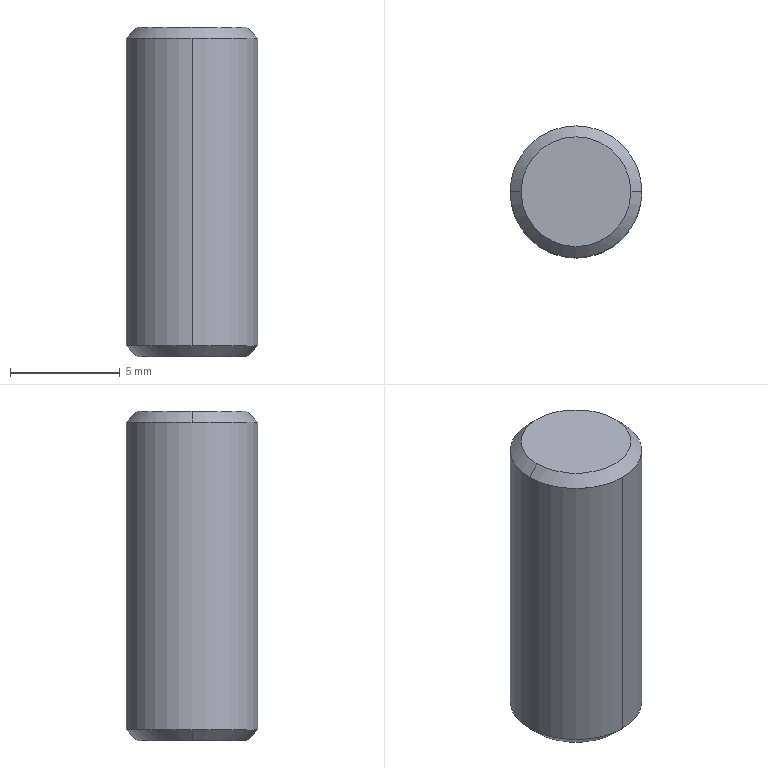Part | SolidWorks | features BaseBody 1 | 1 solid | 8 faces | box 6 x 6 x 15 mm | volume 419.664 mm3 | cone 4 | cylinder 2 | plane 2 | commonest cylinder face diameters 6 x2
STEP:
#1=CARTESIAN_POINT('',(3.,0.,14.5));
#2=VERTEX_POINT('',#1);
#3=CARTESIAN_POINT('',(0.,-3.,14.5));
#4=VERTEX_POINT('',#3);
#5=CARTESIAN_POINT('',(0.,0.,14.5));
#6=DIRECTION('',(0.,0.,-1.));
#7=DIRECTION('',(0.,1.,0.));
#8=AXIS2_PLACEMENT_3D('',#5,#6,#7);
#9=CIRCLE('',#8,3.);
#10=EDGE_CURVE('',#2,#4,#9,.T.);
#11=ORIENTED_EDGE('',*,*,#10,.T.);
#12=CARTESIAN_POINT('',(0.,-3.,0.5));
#13=VERTEX_POINT('',#12);
#14=CARTESIAN_POINT('',(0.,-3.,15.));
#15=DIRECTION('',(0.,0.,-1.));
#16=VECTOR('',#15,1000.);
#17=LINE('',#14,#16);
#18=EDGE_CURVE('',#4,#13,#17,.T.);
#19=ORIENTED_EDGE('',*,*,#18,.T.);
#20=CARTESIAN_POINT('',(3.,0.,0.5));
#21=VERTEX_POINT('',#20);
#22=CARTESIAN_POINT('',(0.,0.,0.5));
#23=DIRECTION('',(0.,0.,1.));
#24=DIRECTION('',(0.,1.,0.));
#25=AXIS2_PLACEMENT_3D('',#22,#23,#24);
#26=CIRCLE('',#25,3.);
#27=EDGE_CURVE('',#13,#21,#26,.T.);
#28=ORIENTED_EDGE('',*,*,#27,.T.);
#29=CARTESIAN_POINT('',(0.,3.,0.5));
#30=VERTEX_POINT('',#29);
#31=CARTESIAN_POINT('',(0.,0.,0.5));
#32=DIRECTION('',(0.,0.,1.));
#33=DIRECTION('',(0.,1.,0.));
#34=AXIS2_PLACEMENT_3D('',#31,#32,#33);
#35=CIRCLE('',#34,3.);
#36=EDGE_CURVE('',#21,#30,#35,.T.);
#37=ORIENTED_EDGE('',*,*,#36,.T.);
#38=CARTESIAN_POINT('',(0.,3.,14.5));
#39=VERTEX_POINT('',#38);
#40=CARTESIAN_POINT('',(0.,3.,15.));
#41=DIRECTION('',(0.,0.,-1.));
#42=VECTOR('',#41,1000.);
#43=LINE('',#40,#42);
#44=EDGE_CURVE('',#39,#30,#43,.T.);
#45=ORIENTED_EDGE('',*,*,#44,.F.);
#46=CARTESIAN_POINT('',(0.,0.,14.5));
#47=DIRECTION('',(0.,0.,-1.));
#48=DIRECTION('',(0.,1.,0.));
#49=AXIS2_PLACEMENT_3D('',#46,#47,#48);
#50=CIRCLE('',#49,3.);
#51=EDGE_CURVE('',#39,#2,#50,.T.);
#52=ORIENTED_EDGE('',*,*,#51,.T.);
#53=EDGE_LOOP('',(#11,#19,#28,#37,#45,#52));
#54=FACE_OUTER_BOUND('',#53,.T.);
#55=CARTESIAN_POINT('',(0.,0.,15.));
#56=DIRECTION('',(0.,0.,-1.));
#57=DIRECTION('',(0.,1.,0.));
#58=AXIS2_PLACEMENT_3D('',#55,#56,#57);
#59=CYLINDRICAL_SURFACE('',#58,3.);
#60=ADVANCED_FACE('',(#54),#59,.T.);
#61=CARTESIAN_POINT('',(2.5,0.,0.));
#62=VERTEX_POINT('',#61);
#63=CARTESIAN_POINT('',(-2.5,0.,0.));
#64=VERTEX_POINT('',#63);
#65=CARTESIAN_POINT('',(0.,0.,0.));
#66=DIRECTION('',(0.,0.,1.));
#67=DIRECTION('',(1.,0.,0.));
#68=AXIS2_PLACEMENT_3D('',#65,#66,#67);
#69=CIRCLE('',#68,2.5);
#70=EDGE_CURVE('',#62,#64,#69,.T.);
#71=ORIENTED_EDGE('',*,*,#70,.T.);
#72=CARTESIAN_POINT('',(-3.,0.,0.5));
#73=VERTEX_POINT('',#72);
#74=CARTESIAN_POINT('',(-3.,0.,0.5));
#75=DIRECTION('',(-0.7071,0.,0.7071));
#76=VECTOR('',#75,1000.);
#77=LINE('',#74,#76);
#78=EDGE_CURVE('',#64,#73,#77,.T.);
#79=ORIENTED_EDGE('',*,*,#78,.T.);
#80=CARTESIAN_POINT('',(0.,0.,0.5));
#81=DIRECTION('',(0.,0.,1.));
#82=DIRECTION('',(0.,1.,0.));
#83=AXIS2_PLACEMENT_3D('',#80,#81,#82);
#84=CIRCLE('',#83,3.);
#85=EDGE_CURVE('',#30,#73,#84,.T.);
#86=ORIENTED_EDGE('',*,*,#85,.F.);
#87=ORIENTED_EDGE('',*,*,#36,.F.);
#88=CARTESIAN_POINT('',(3.,0.,0.5));
#89=DIRECTION('',(0.7071,0.,0.7071));
#90=VECTOR('',#89,1000.);
#91=LINE('',#88,#90);
#92=EDGE_CURVE('',#62,#21,#91,.T.);
#93=ORIENTED_EDGE('',*,*,#92,.F.);
#94=EDGE_LOOP('',(#71,#79,#86,#87,#93));
#95=FACE_OUTER_BOUND('',#94,.T.);
#96=CARTESIAN_POINT('',(0.,0.,0.5));
#97=DIRECTION('',(0.,0.,1.));
#98=DIRECTION('',(1.,0.,0.));
#99=AXIS2_PLACEMENT_3D('',#96,#97,#98);
#100=CONICAL_SURFACE('',#99,3.,0.7854);
#101=ADVANCED_FACE('',(#95),#100,.T.);
#102=CARTESIAN_POINT('',(-2.5,0.,15.));
#103=VERTEX_POINT('',#102);
#104=CARTESIAN_POINT('',(2.5,0.,15.));
#105=VERTEX_POINT('',#104);
#106=CARTESIAN_POINT('',(0.,0.,15.));
#107=DIRECTION('',(0.,0.,-1.));
#108=DIRECTION('',(-1.,0.,0.));
#109=AXIS2_PLACEMENT_3D('',#106,#107,#108);
#110=CIRCLE('',#109,2.5);
#111=EDGE_CURVE('',#103,#105,#110,.T.);
#112=ORIENTED_EDGE('',*,*,#111,.T.);
#113=CARTESIAN_POINT('',(3.,0.,14.5));
#114=DIRECTION('',(0.7071,0.,-0.7071));
#115=VECTOR('',#114,1000.);
#116=LINE('',#113,#115);
#117=EDGE_CURVE('',#105,#2,#116,.T.);
#118=ORIENTED_EDGE('',*,*,#117,.T.);
#119=ORIENTED_EDGE('',*,*,#51,.F.);
#120=CARTESIAN_POINT('',(-3.,0.,14.5));
#121=VERTEX_POINT('',#120);
#122=CARTESIAN_POINT('',(0.,0.,14.5));
#123=DIRECTION('',(0.,0.,-1.));
#124=DIRECTION('',(0.,1.,0.));
#125=AXIS2_PLACEMENT_3D('',#122,#123,#124);
#126=CIRCLE('',#125,3.);
#127=EDGE_CURVE('',#121,#39,#126,.T.);
#128=ORIENTED_EDGE('',*,*,#127,.F.);
#129=CARTESIAN_POINT('',(-3.,0.,14.5));
#130=DIRECTION('',(-0.7071,0.,-0.7071));
#131=VECTOR('',#130,1000.);
#132=LINE('',#129,#131);
#133=EDGE_CURVE('',#103,#121,#132,.T.);
#134=ORIENTED_EDGE('',*,*,#133,.F.);
#135=EDGE_LOOP('',(#112,#118,#119,#128,#134));
#136=FACE_OUTER_BOUND('',#135,.T.);
#137=CARTESIAN_POINT('',(0.,0.,14.5));
#138=DIRECTION('',(0.,0.,-1.));
#139=DIRECTION('',(-1.,0.,0.));
#140=AXIS2_PLACEMENT_3D('',#137,#138,#139);
#141=CONICAL_SURFACE('',#140,3.,0.7854);
#142=ADVANCED_FACE('',(#136),#141,.T.);
#143=ORIENTED_EDGE('',*,*,#18,.F.);
#144=CARTESIAN_POINT('',(0.,0.,14.5));
#145=DIRECTION('',(0.,0.,-1.));
#146=DIRECTION('',(0.,1.,0.));
#147=AXIS2_PLACEMENT_3D('',#144,#145,#146);
#148=CIRCLE('',#147,3.);
#149=EDGE_CURVE('',#4,#121,#148,.T.);
#150=ORIENTED_EDGE('',*,*,#149,.T.);
#151=ORIENTED_EDGE('',*,*,#127,.T.);
#152=ORIENTED_EDGE('',*,*,#44,.T.);
#153=ORIENTED_EDGE('',*,*,#85,.T.);
#154=CARTESIAN_POINT('',(0.,0.,0.5));
#155=DIRECTION('',(0.,0.,1.));
#156=DIRECTION('',(0.,1.,0.));
#157=AXIS2_PLACEMENT_3D('',#154,#155,#156);
#158=CIRCLE('',#157,3.);
#159=EDGE_CURVE('',#73,#13,#158,.T.);
#160=ORIENTED_EDGE('',*,*,#159,.T.);
#161=EDGE_LOOP('',(#143,#150,#151,#152,#153,#160));
#162=FACE_OUTER_BOUND('',#161,.T.);
#163=CARTESIAN_POINT('',(0.,0.,15.));
#164=DIRECTION('',(0.,0.,-1.));
#165=DIRECTION('',(0.,1.,0.));
#166=AXIS2_PLACEMENT_3D('',#163,#164,#165);
#167=CYLINDRICAL_SURFACE('',#166,3.);
#168=ADVANCED_FACE('',(#162),#167,.T.);
#169=ORIENTED_EDGE('',*,*,#78,.F.);
#170=CARTESIAN_POINT('',(0.,0.,0.));
#171=DIRECTION('',(0.,0.,1.));
#172=DIRECTION('',(1.,0.,0.));
#173=AXIS2_PLACEMENT_3D('',#170,#171,#172);
#174=CIRCLE('',#173,2.5);
#175=EDGE_CURVE('',#64,#62,#174,.T.);
#176=ORIENTED_EDGE('',*,*,#175,.T.);
#177=ORIENTED_EDGE('',*,*,#92,.T.);
#178=ORIENTED_EDGE('',*,*,#27,.F.);
#179=ORIENTED_EDGE('',*,*,#159,.F.);
#180=EDGE_LOOP('',(#169,#176,#177,#178,#179));
#181=FACE_OUTER_BOUND('',#180,.T.);
#182=CARTESIAN_POINT('',(0.,0.,0.5));
#183=DIRECTION('',(0.,0.,1.));
#184=DIRECTION('',(1.,0.,0.));
#185=AXIS2_PLACEMENT_3D('',#182,#183,#184);
#186=CONICAL_SURFACE('',#185,3.,0.7854);
#187=ADVANCED_FACE('',(#181),#186,.T.);
#188=ORIENTED_EDGE('',*,*,#117,.F.);
#189=CARTESIAN_POINT('',(0.,0.,15.));
#190=DIRECTION('',(0.,0.,-1.));
#191=DIRECTION('',(-1.,0.,0.));
#192=AXIS2_PLACEMENT_3D('',#189,#190,#191);
#193=CIRCLE('',#192,2.5);
#194=EDGE_CURVE('',#105,#103,#193,.T.);
#195=ORIENTED_EDGE('',*,*,#194,.T.);
#196=ORIENTED_EDGE('',*,*,#133,.T.);
#197=ORIENTED_EDGE('',*,*,#149,.F.);
#198=ORIENTED_EDGE('',*,*,#10,.F.);
#199=EDGE_LOOP('',(#188,#195,#196,#197,#198));
#200=FACE_OUTER_BOUND('',#199,.T.);
#201=CARTESIAN_POINT('',(0.,0.,14.5));
#202=DIRECTION('',(0.,0.,-1.));
#203=DIRECTION('',(-1.,0.,0.));
#204=AXIS2_PLACEMENT_3D('',#201,#202,#203);
#205=CONICAL_SURFACE('',#204,3.,0.7854);
#206=ADVANCED_FACE('',(#200),#205,.T.);
#207=ORIENTED_EDGE('',*,*,#70,.F.);
#208=ORIENTED_EDGE('',*,*,#175,.F.);
#209=EDGE_LOOP('',(#207,#208));
#210=FACE_OUTER_BOUND('',#209,.T.);
#211=CARTESIAN_POINT('',(0.,0.,0.));
#212=DIRECTION('',(0.,0.,1.));
#213=DIRECTION('',(0.,-1.,0.));
#214=AXIS2_PLACEMENT_3D('',#211,#212,#213);
#215=PLANE('',#214);
#216=ADVANCED_FACE('',(#210),#215,.F.);
#217=ORIENTED_EDGE('',*,*,#111,.F.);
#218=ORIENTED_EDGE('',*,*,#194,.F.);
#219=EDGE_LOOP('',(#217,#218));
#220=FACE_OUTER_BOUND('',#219,.T.);
#221=CARTESIAN_POINT('',(0.,0.,15.));
#222=DIRECTION('',(0.,0.,1.));
#223=DIRECTION('',(0.,-1.,0.));
#224=AXIS2_PLACEMENT_3D('',#221,#222,#223);
#225=PLANE('',#224);
#226=ADVANCED_FACE('',(#220),#225,.T.);
#227=CLOSED_SHELL('',(#60,#101,#142,#168,#187,#206,#216,#226));
#228=MANIFOLD_SOLID_BREP('',#227);
#229=CARTESIAN_POINT('',(0.,0.,0.));
#230=DIRECTION('',(0.,0.,1.));
#231=DIRECTION('',(1.,0.,0.));
#232=AXIS2_PLACEMENT_3D('',#229,#230,#231);
#233=(LENGTH_UNIT()NAMED_UNIT(*)SI_UNIT(.MILLI.,.METRE.));
#234=UNCERTAINTY_MEASURE_WITH_UNIT(LENGTH_MEASURE(0.00001),#233,'','');
#235=(NAMED_UNIT(*)PLANE_ANGLE_UNIT()SI_UNIT($,.RADIAN.));
#236=(NAMED_UNIT(*)SI_UNIT($,.STERADIAN.)SOLID_ANGLE_UNIT());
#237=(GEOMETRIC_REPRESENTATION_CONTEXT(3)GLOBAL_UNCERTAINTY_ASSIGNED_CONTEXT((#234))GLOBAL_UNIT_ASSIGNED_CONTEXT((#233,#235,#236))REPRESENTATION_CONTEXT('',''));
#238=ADVANCED_BREP_SHAPE_REPRESENTATION('',(#228,#232),#237);